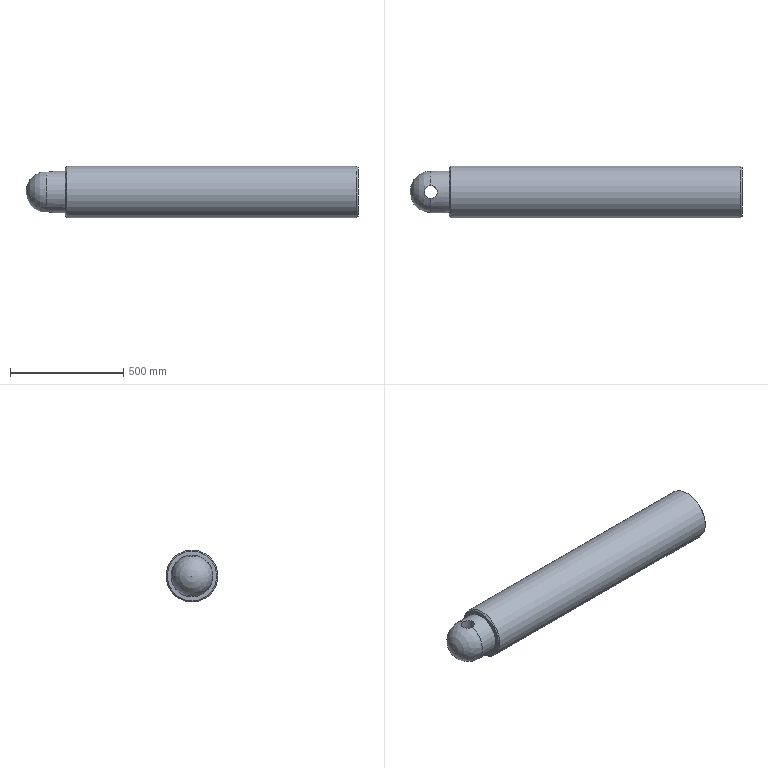Part | NX | features 立柱活塞 2 | 1 solid | 8 faces | box 1466 x 228.3 x 228.3 mm | volume 56225890 mm3 | cylinder 3 | plane 2 | cone 2 | sphere 1 | commonest cylinder face diameters 56.58 x1 184 x1 228.3 x1
STEP:
#1=CARTESIAN_POINT('',(-142.24,0.,109.15));
#2=VERTEX_POINT('',#1);
#3=CARTESIAN_POINT('',(-142.24,0.,0.));
#4=DIRECTION('',(-1.,0.,0.));
#5=DIRECTION('',(0.,0.,1.));
#6=AXIS2_PLACEMENT_3D('',#3,#4,#5);
#7=CIRCLE('',#6,109.15);
#8=EDGE_CURVE('',#2,#2,#7,.T.);
#9=ORIENTED_EDGE('',*,*,#8,.T.);
#10=EDGE_LOOP('',(#9));
#11=FACE_BOUND('',#10,.T.);
#12=CARTESIAN_POINT('',(-142.24,0.,92.));
#13=VERTEX_POINT('',#12);
#14=CARTESIAN_POINT('',(-142.24,0.,0.));
#15=DIRECTION('',(-1.,0.,0.));
#16=DIRECTION('',(0.,0.,1.));
#17=AXIS2_PLACEMENT_3D('',#14,#15,#16);
#18=CIRCLE('',#17,92.);
#19=EDGE_CURVE('',#13,#13,#18,.T.);
#20=ORIENTED_EDGE('',*,*,#19,.F.);
#21=EDGE_LOOP('',(#20));
#22=FACE_BOUND('',#21,.T.);
#23=CARTESIAN_POINT('',(-142.24,-114.15,0.));
#24=DIRECTION('',(-1.,0.,0.));
#25=DIRECTION('',(0.,0.,1.));
#26=AXIS2_PLACEMENT_3D('',#23,#24,#25);
#27=PLANE('',#26);
#28=ADVANCED_FACE('',(#11,#22),#27,.T.);
#29=CARTESIAN_POINT('',(1144.704,0.,-114.15));
#30=VERTEX_POINT('',#29);
#31=CARTESIAN_POINT('',(1144.704,0.,0.));
#32=DIRECTION('',(1.,0.,0.));
#33=DIRECTION('',(0.,0.,-1.));
#34=AXIS2_PLACEMENT_3D('',#31,#32,#33);
#35=CIRCLE('',#34,114.15);
#36=EDGE_CURVE('',#30,#30,#35,.F.);
#37=ORIENTED_EDGE('',*,*,#36,.T.);
#38=EDGE_LOOP('',(#37));
#39=FACE_BOUND('',#38,.T.);
#40=CARTESIAN_POINT('',(-137.24,0.,114.15));
#41=VERTEX_POINT('',#40);
#42=CARTESIAN_POINT('',(-137.24,0.,0.));
#43=DIRECTION('',(-1.,0.,0.));
#44=DIRECTION('',(0.,0.,1.));
#45=AXIS2_PLACEMENT_3D('',#42,#43,#44);
#46=CIRCLE('',#45,114.15);
#47=EDGE_CURVE('',#41,#41,#46,.F.);
#48=ORIENTED_EDGE('',*,*,#47,.T.);
#49=EDGE_LOOP('',(#48));
#50=FACE_BOUND('',#49,.T.);
#51=CARTESIAN_POINT('',(-316.24,0.,0.));
#52=DIRECTION('',(-1.,0.,0.));
#53=DIRECTION('',(0.,0.,1.));
#54=AXIS2_PLACEMENT_3D('',#51,#52,#53);
#55=CYLINDRICAL_SURFACE('',#54,114.15);
#56=ADVANCED_FACE('',(#39,#50),#55,.T.);
#57=CARTESIAN_POINT('',(1149.704,0.,-109.15));
#58=VERTEX_POINT('',#57);
#59=CARTESIAN_POINT('',(1149.704,0.,0.));
#60=DIRECTION('',(1.,0.,0.));
#61=DIRECTION('',(0.,0.,-1.));
#62=AXIS2_PLACEMENT_3D('',#59,#60,#61);
#63=CIRCLE('',#62,109.15);
#64=EDGE_CURVE('',#58,#58,#63,.T.);
#65=ORIENTED_EDGE('',*,*,#64,.T.);
#66=EDGE_LOOP('',(#65));
#67=FACE_BOUND('',#66,.T.);
#68=CARTESIAN_POINT('',(1149.704,-114.15,0.));
#69=DIRECTION('',(1.,0.,0.));
#70=DIRECTION('',(0.,0.,-1.));
#71=AXIS2_PLACEMENT_3D('',#68,#69,#70);
#72=PLANE('',#71);
#73=ADVANCED_FACE('',(#67),#72,.T.);
#74=CARTESIAN_POINT('',(-224.24,28.29,87.542));
#75=VERTEX_POINT('',#74);
#76=CARTESIAN_POINT('',(-224.24,-28.29,87.542));
#77=VERTEX_POINT('',#76);
#78=CARTESIAN_POINT('',(-224.24,0.,87.542));
#79=DIRECTION('',(0.,0.,-1.));
#80=DIRECTION('',(-1.,0.,0.));
#81=AXIS2_PLACEMENT_3D('',#78,#79,#80);
#82=CIRCLE('',#81,28.29);
#83=EDGE_CURVE('',#75,#77,#82,.F.);
#84=ORIENTED_EDGE('',*,*,#83,.F.);
#85=CARTESIAN_POINT('',(-224.24,28.29,-87.542));
#86=VERTEX_POINT('',#85);
#87=CARTESIAN_POINT('',(-224.24,0.,0.));
#88=DIRECTION('',(-1.,0.,0.));
#89=DIRECTION('',(0.,0.,1.));
#90=AXIS2_PLACEMENT_3D('',#87,#88,#89);
#91=CIRCLE('',#90,92.);
#92=EDGE_CURVE('',#75,#86,#91,.T.);
#93=ORIENTED_EDGE('',*,*,#92,.T.);
#94=CARTESIAN_POINT('',(-224.24,-28.29,-87.542));
#95=VERTEX_POINT('',#94);
#96=CARTESIAN_POINT('',(-224.24,0.,-87.542));
#97=DIRECTION('',(0.,0.,1.));
#98=DIRECTION('',(1.,0.,0.));
#99=AXIS2_PLACEMENT_3D('',#96,#97,#98);
#100=CIRCLE('',#99,28.29);
#101=EDGE_CURVE('',#95,#86,#100,.F.);
#102=ORIENTED_EDGE('',*,*,#101,.F.);
#103=CARTESIAN_POINT('',(-224.24,0.,0.));
#104=DIRECTION('',(-1.,0.,0.));
#105=DIRECTION('',(0.,0.,1.));
#106=AXIS2_PLACEMENT_3D('',#103,#104,#105);
#107=CIRCLE('',#106,92.);
#108=EDGE_CURVE('',#95,#77,#107,.T.);
#109=ORIENTED_EDGE('',*,*,#108,.T.);
#110=EDGE_LOOP('',(#84,#93,#102,#109));
#111=FACE_BOUND('',#110,.T.);
#112=CARTESIAN_POINT('',(-224.24,0.,0.));
#113=DIRECTION('',(-1.,0.,0.));
#114=DIRECTION('',(0.,1.,0.));
#115=AXIS2_PLACEMENT_3D('',#112,#113,#114);
#116=SPHERICAL_SURFACE('',#115,92.);
#117=ADVANCED_FACE('',(#111),#116,.T.);
#118=CARTESIAN_POINT('',(-224.24,-28.29,87.542));
#119=CARTESIAN_POINT('',(-222.359,-28.29,87.542));
#120=CARTESIAN_POINT('',(-218.672,-27.923,87.662));
#121=CARTESIAN_POINT('',(-211.496,-25.738,88.345));
#122=CARTESIAN_POINT('',(-203.73,-20.517,89.804));
#123=CARTESIAN_POINT('',(-197.455,-11.181,91.521));
#124=CARTESIAN_POINT('',(-195.202,-0.03347,92.238));
#125=CARTESIAN_POINT('',(-197.435,11.145,91.527));
#126=CARTESIAN_POINT('',(-203.72,20.516,89.806));
#127=CARTESIAN_POINT('',(-213.063,26.781,88.05));
#128=CARTESIAN_POINT('',(-220.478,28.29,87.542));
#129=CARTESIAN_POINT('',(-224.24,28.29,87.542));
#130=B_SPLINE_CURVE_WITH_KNOTS('',3,(#118,#119,#120,#121,#122,#123,#124,#125,#126,#127,#128,#129),.UNSPECIFIED.,.F.,.F.,(4,1,1,1,1,1,1,1,1,4),(0.,0.00556,0.01112,0.02224,0.03336,0.04448,0.0556,0.06672,0.07784,0.08896),.UNSPECIFIED.);
#131=EDGE_CURVE('',#77,#75,#130,.T.);
#132=ORIENTED_EDGE('',*,*,#131,.F.);
#133=ORIENTED_EDGE('',*,*,#108,.F.);
#134=CARTESIAN_POINT('',(-224.24,28.29,-87.542));
#135=CARTESIAN_POINT('',(-222.359,28.29,-87.542));
#136=CARTESIAN_POINT('',(-218.672,27.923,-87.662));
#137=CARTESIAN_POINT('',(-211.496,25.738,-88.345));
#138=CARTESIAN_POINT('',(-203.73,20.517,-89.804));
#139=CARTESIAN_POINT('',(-197.455,11.181,-91.521));
#140=CARTESIAN_POINT('',(-195.202,0.03347,-92.238));
#141=CARTESIAN_POINT('',(-197.435,-11.145,-91.527));
#142=CARTESIAN_POINT('',(-203.72,-20.516,-89.806));
#143=CARTESIAN_POINT('',(-213.063,-26.781,-88.05));
#144=CARTESIAN_POINT('',(-220.478,-28.29,-87.542));
#145=CARTESIAN_POINT('',(-224.24,-28.29,-87.542));
#146=B_SPLINE_CURVE_WITH_KNOTS('',3,(#134,#135,#136,#137,#138,#139,#140,#141,#142,#143,#144,#145),.UNSPECIFIED.,.F.,.F.,(4,1,1,1,1,1,1,1,1,4),(0.,0.00556,0.01112,0.02224,0.03336,0.04448,0.0556,0.06672,0.07784,0.08896),.UNSPECIFIED.);
#147=EDGE_CURVE('',#86,#95,#146,.T.);
#148=ORIENTED_EDGE('',*,*,#147,.F.);
#149=ORIENTED_EDGE('',*,*,#92,.F.);
#150=EDGE_LOOP('',(#132,#133,#148,#149));
#151=FACE_BOUND('',#150,.T.);
#152=ORIENTED_EDGE('',*,*,#19,.T.);
#153=EDGE_LOOP('',(#152));
#154=FACE_BOUND('',#153,.T.);
#155=CARTESIAN_POINT('',(-316.24,0.,0.));
#156=DIRECTION('',(-1.,0.,0.));
#157=DIRECTION('',(0.,0.,1.));
#158=AXIS2_PLACEMENT_3D('',#155,#156,#157);
#159=CYLINDRICAL_SURFACE('',#158,92.);
#160=ADVANCED_FACE('',(#151,#154),#159,.T.);
#161=ORIENTED_EDGE('',*,*,#83,.T.);
#162=ORIENTED_EDGE('',*,*,#131,.T.);
#163=EDGE_LOOP('',(#161,#162));
#164=FACE_BOUND('',#163,.T.);
#165=ORIENTED_EDGE('',*,*,#101,.T.);
#166=ORIENTED_EDGE('',*,*,#147,.T.);
#167=EDGE_LOOP('',(#165,#166));
#168=FACE_BOUND('',#167,.T.);
#169=CARTESIAN_POINT('',(-224.24,0.,-100.));
#170=DIRECTION('',(0.,0.,1.));
#171=DIRECTION('',(1.,0.,0.));
#172=AXIS2_PLACEMENT_3D('',#169,#170,#171);
#173=CYLINDRICAL_SURFACE('',#172,28.29);
#174=ADVANCED_FACE('',(#164,#168),#173,.F.);
#175=ORIENTED_EDGE('',*,*,#47,.F.);
#176=EDGE_LOOP('',(#175));
#177=FACE_BOUND('',#176,.T.);
#178=ORIENTED_EDGE('',*,*,#8,.F.);
#179=EDGE_LOOP('',(#178));
#180=FACE_BOUND('',#179,.T.);
#181=CARTESIAN_POINT('',(-142.24,0.,0.));
#182=DIRECTION('',(1.,0.,0.));
#183=DIRECTION('',(0.,0.,-1.));
#184=AXIS2_PLACEMENT_3D('',#181,#182,#183);
#185=CONICAL_SURFACE('',#184,109.15,0.7854);
#186=ADVANCED_FACE('',(#177,#180),#185,.T.);
#187=ORIENTED_EDGE('',*,*,#64,.F.);
#188=EDGE_LOOP('',(#187));
#189=FACE_BOUND('',#188,.T.);
#190=ORIENTED_EDGE('',*,*,#36,.F.);
#191=EDGE_LOOP('',(#190));
#192=FACE_BOUND('',#191,.T.);
#193=CARTESIAN_POINT('',(1144.704,0.,0.));
#194=DIRECTION('',(-1.,0.,0.));
#195=DIRECTION('',(0.,0.,1.));
#196=AXIS2_PLACEMENT_3D('',#193,#194,#195);
#197=CONICAL_SURFACE('',#196,114.15,0.7854);
#198=ADVANCED_FACE('',(#189,#192),#197,.T.);
#199=CLOSED_SHELL('',(#28,#56,#73,#117,#160,#174,#186,#198));
#200=MANIFOLD_SOLID_BREP('',#199);
#201=(LENGTH_UNIT()NAMED_UNIT(*)SI_UNIT(.MILLI.,.METRE.));
#202=UNCERTAINTY_MEASURE_WITH_UNIT(LENGTH_MEASURE(0.0508),#201,'','');
#203=(NAMED_UNIT(*)PLANE_ANGLE_UNIT()SI_UNIT($,.RADIAN.));
#204=(NAMED_UNIT(*)SI_UNIT($,.STERADIAN.)SOLID_ANGLE_UNIT());
#205=(GEOMETRIC_REPRESENTATION_CONTEXT(3)GLOBAL_UNCERTAINTY_ASSIGNED_CONTEXT((#202))GLOBAL_UNIT_ASSIGNED_CONTEXT((#201,#203,#204))REPRESENTATION_CONTEXT('',''));
#206=ADVANCED_BREP_SHAPE_REPRESENTATION('',(#200),#205);